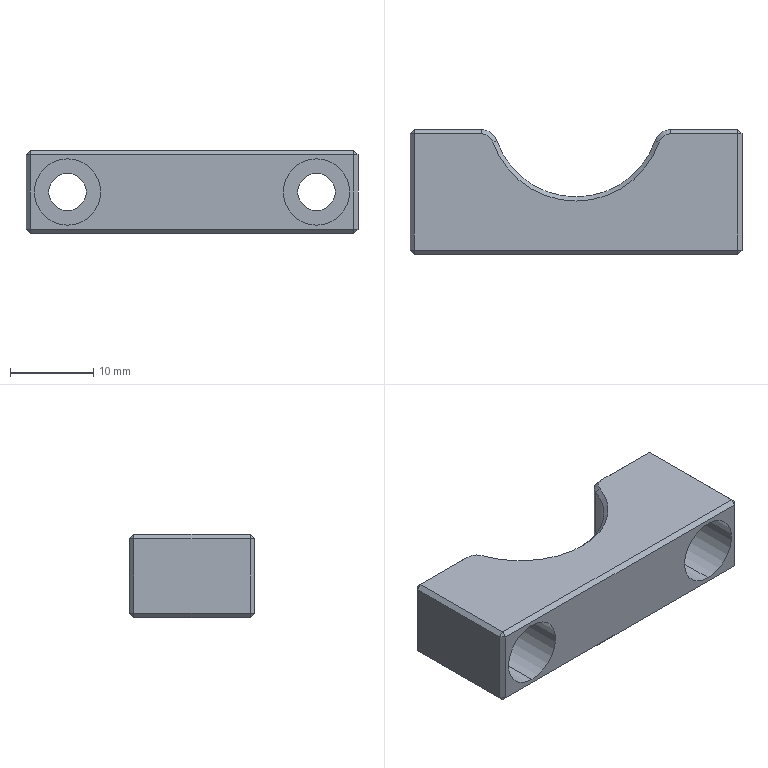Part | STEP file | photoelectric switch fixing block 1 | 1 solid | 48 faces | box 40 x 15 x 10 mm | volume 3490 mm3 | plane 31 | cylinder 11 | cone 6 | commonest cylinder face diameters 4.5 x4 8 x4 4 x2 20.2 x1